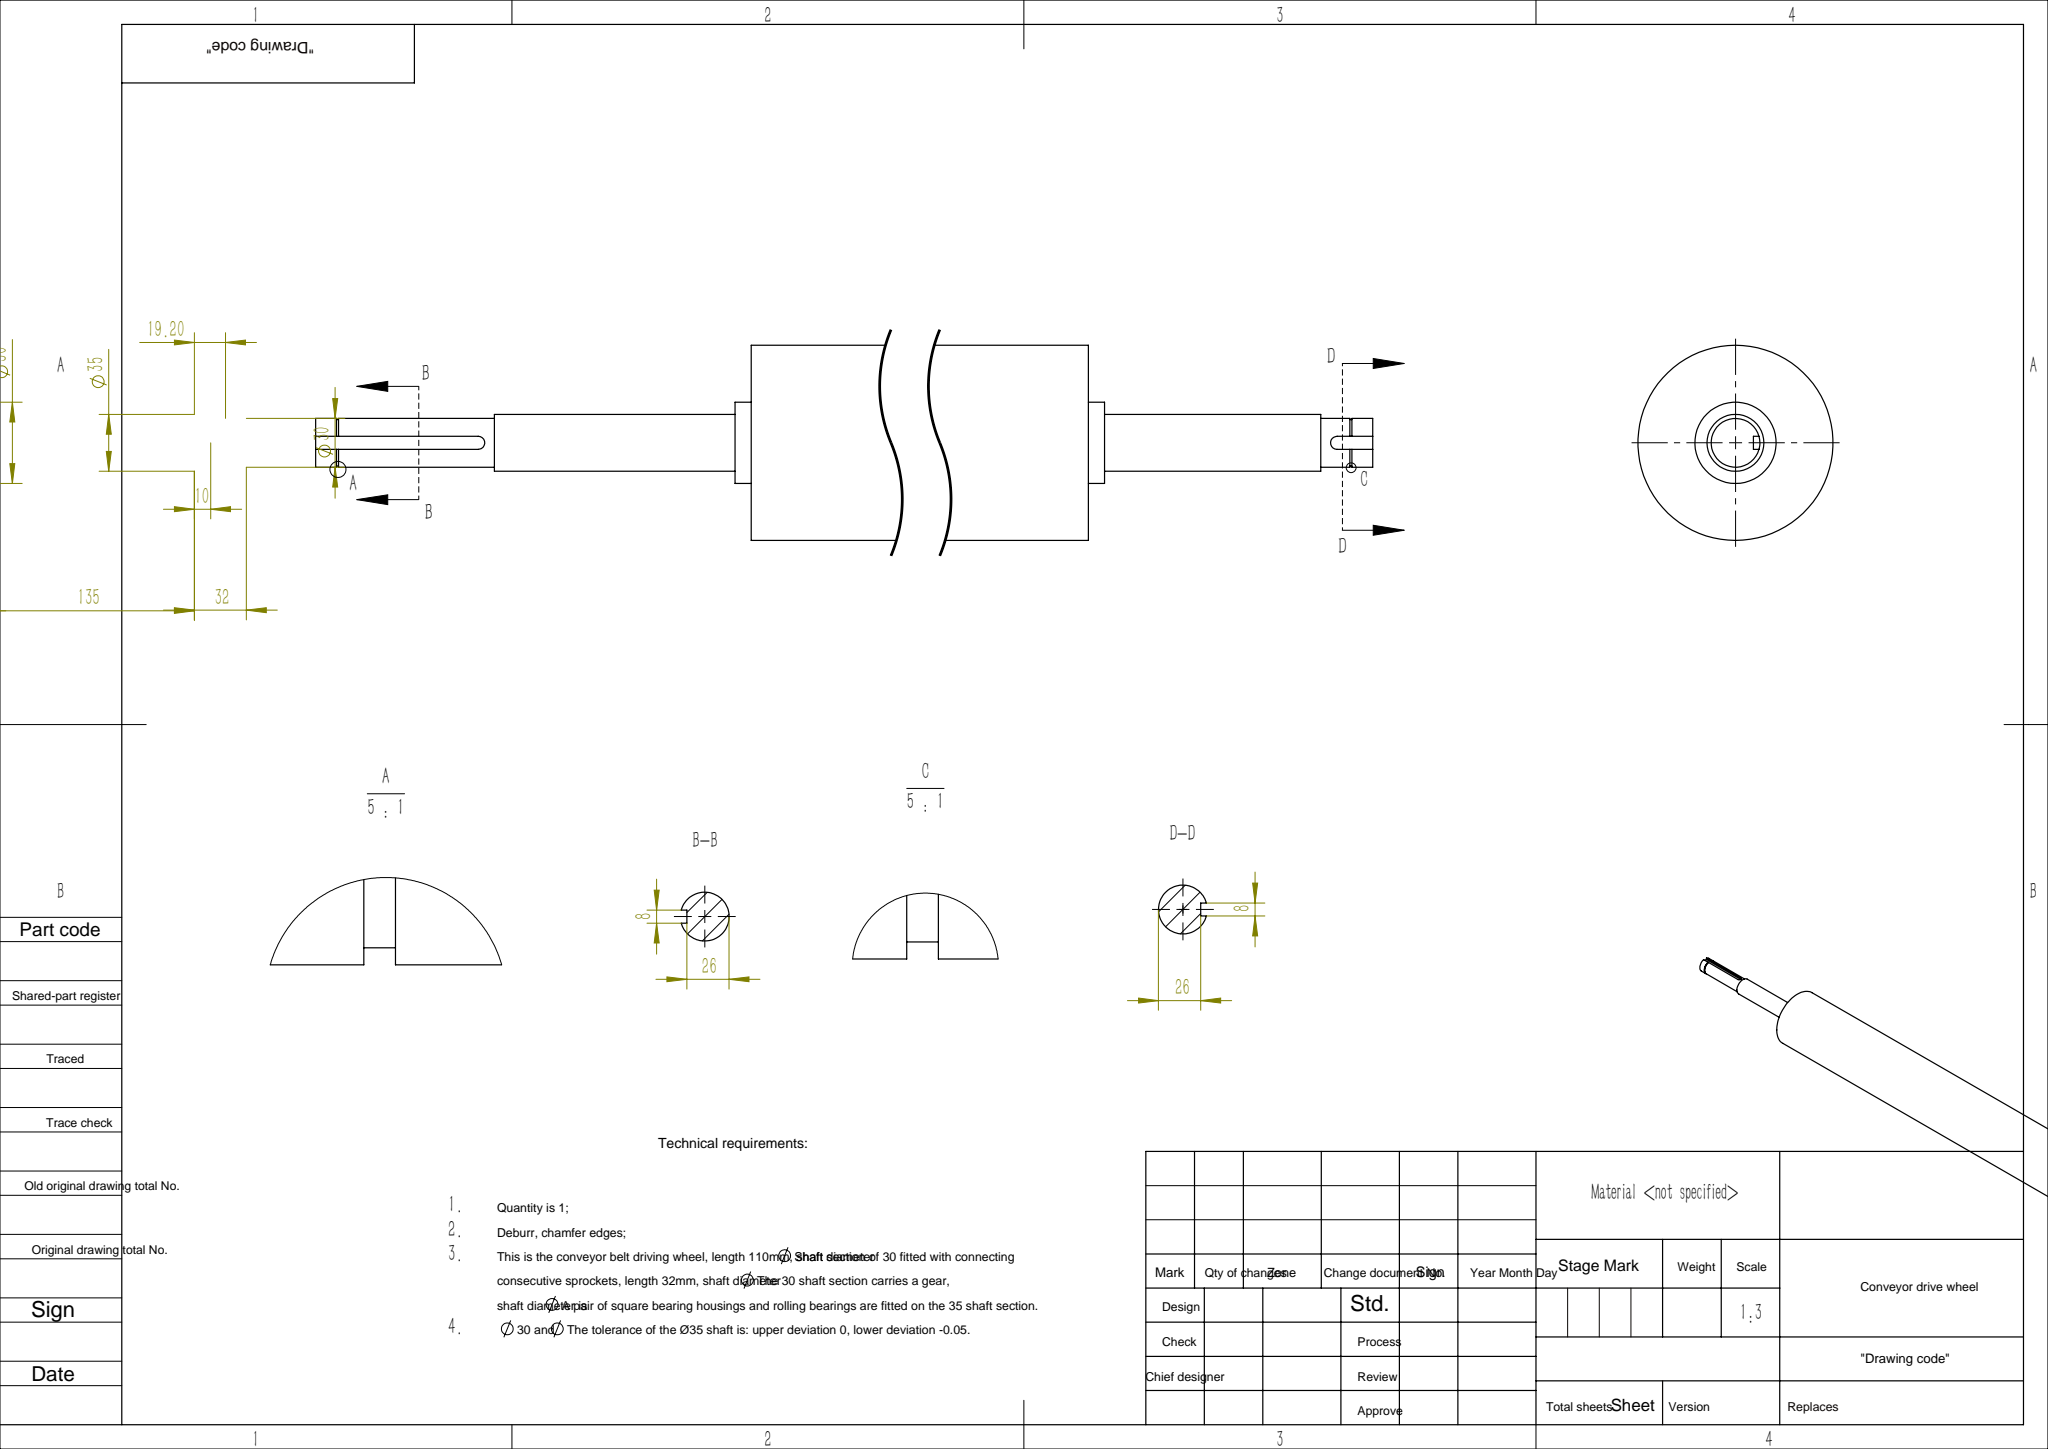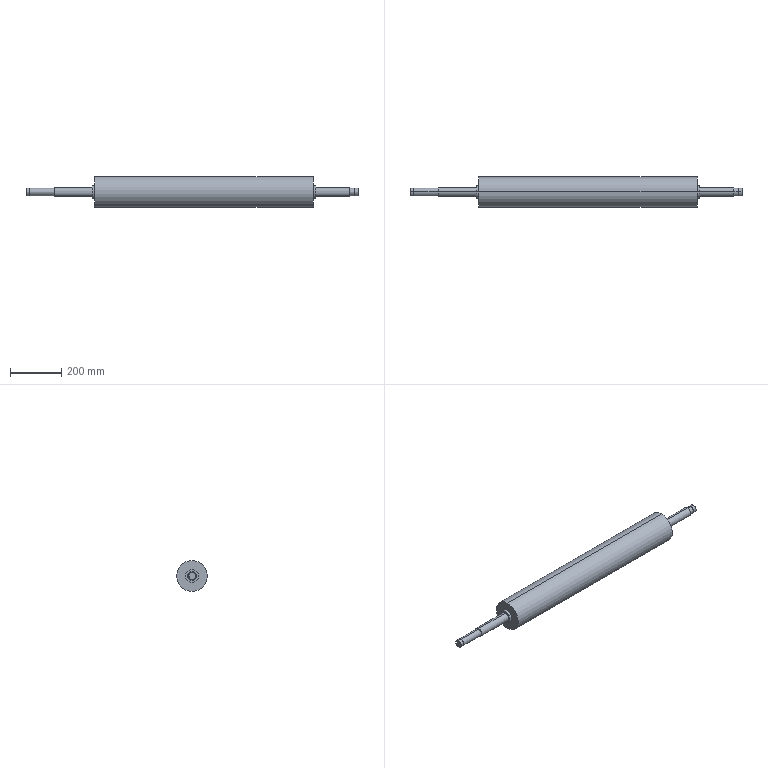Part | SolidWorks | features ICE 4, Revolution 1 | 1 solid | 46 faces | box 1293 x 120 x 120 mm | volume 10019195 mm3 | cylinder 28 | plane 18 | commonest cylinder face diameters 30 x10 28.6 x6 35 x4 50 x4 8 x2 120 x2